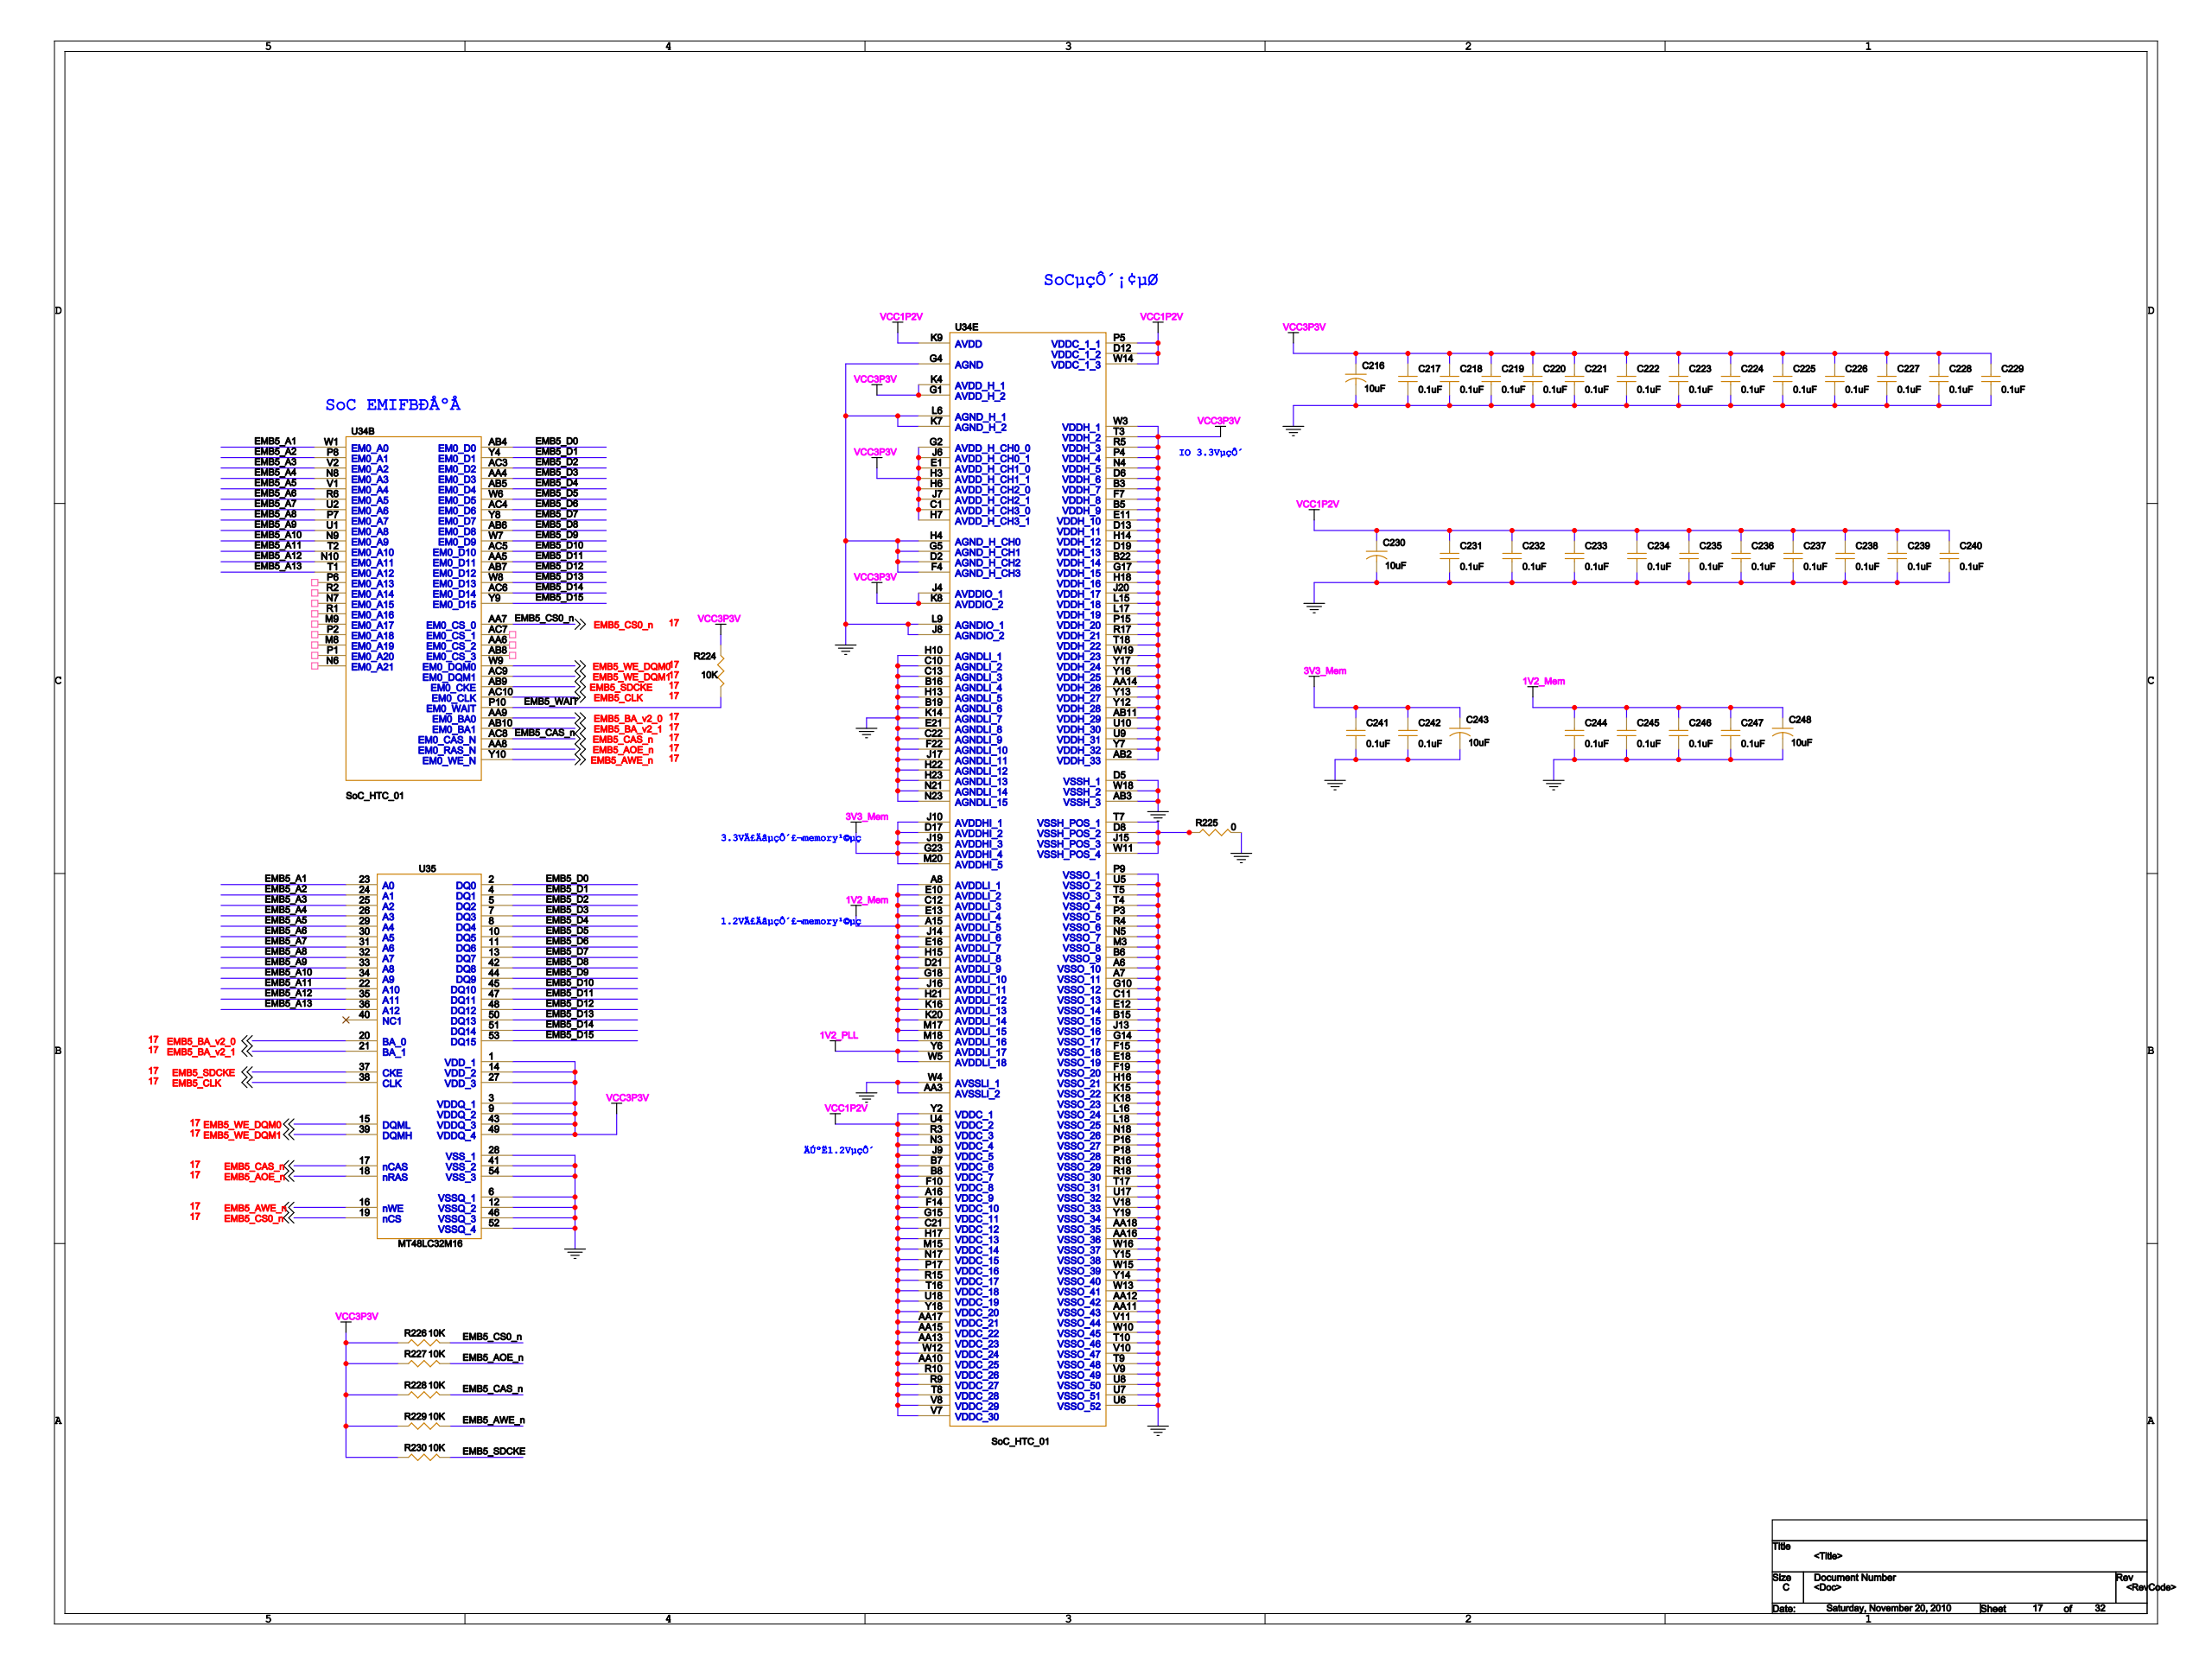Circuit board | Cadence Allegro | 1001 parts | 1318 nets | one sheet of the schematic
Parts on this sheet (reference | value | footprint):
C216 | 10uF | C3216
C217 | 0.1uF | C0402
C218 | 0.1uF | C0402
C219 | 0.1uF | C0402
C220 | 0.1uF | C0402
C221 | 0.1uF | C0402
C222 | 0.1uF | C0402
C223 | 0.1uF | C0402
C224 | 0.1uF | C0402
C225 | 0.1uF | C0402
C226 | 0.1uF | C0402
C227 | 0.1uF | C0402
C228 | 0.1uF | C0402
C229 | 0.1uF | C0402
C230 | 10uF | C3216
C231 | 0.1uF | C0402
C232 | 0.1uF | C0402
C233 | 0.1uF | C0402
C234 | 0.1uF | C0402
C235 | 0.1uF | C0402
C236 | 0.1uF | C0402
C237 | 0.1uF | C0402
C238 | 0.1uF | C0402
C239 | 0.1uF | C0402
C240 | 0.1uF | C0402
C241 | 0.1uF | C0402
C242 | 0.1uF | C0402
C243 | 10uF | C3216
C244 | 0.1uF | C0402
C245 | 0.1uF | C0402
C246 | 0.1uF | C0402
C247 | 0.1uF | C0402
C248 | 10uF | C3216
R224 | 10K | 0603
R225 | 0 | 0603
R226 | 10K | 0603
R227 | 10K | 0603
R228 | 10K | 0603
R229 | 10K | 0603
R230 | 10K | 0603
U1 | SoC_HTC_01 | L529_XIN
U2 | MT48LC32M16 | TSOP54
U4 | MAX3243 | TSSOP-28
U6 | MT48LC16M16 | TSOP54
U7 | MT48LC16M16 | TSOP54
U8 | DP83848C | DP83848C_48LQFP
U10 | SoC_HTC_01 | L529_XIN
U17 | MT48LC32M16 | TSOP54
U34 | SoC_HTC_01 | L529_XIN
U35 | MT48LC32M16 | TSOP54
Nets of these parts (net: part-pin ...):
GND: C216-2 C217-2 C218-2 C219-2 C220-2 C221-2 C222-2 C223-2 C224-2 C225-2 C226-2 C227-2 C228-2 C229-2 C230-2 C231-2 C232-2 C233-2 C234-2 C235-2 C236-2 C237-2 C238-2 C239-2 C240-2 C241-2 C242-2 C243-2 C244-2 C245-2 C246-2 C247-2 C248-2 R225-2 U1-A6 U1-A7 U1-AA3 U1-AA11 U1-AA12 U1-AA16 U1-AA18 U1-AB3 U1-B6 U1-B15 U1-B16 U1-B19 U1-C10 U1-C11 U1-C13 U1-C22 U1-D2 U1-D5 U1-E12 U1-E18 U1-E21 U1-F4 U1-F15 U1-F19 U1-F22 U1-G4 U1-G5 U1-G10 U1-G14 U1-H4 U1-H10 U1-H13 U1-H16 U1-H22 U1-H23 U1-J8 U1-J13 U1-J17 U1-K7 U1-K14 U1-K15 U1-K18 U1-L6 U1-L9 U1-L16 U1-L18 U1-M3 U1-N5 U1-N18 U1-N21 U1-N23 U1-P3 U1-P9 U1-P16 U1-P18 U1-R4 U1-R16 U1-R18 U1-T4 U1-T5 U1-T9 U1-T10 U1-T17 U1-U5 U1-U6 U1-U7 U1-U8 U1-U17 U1-V9 U1-V10 U1-V11 U1-V18 U1-W4 U1-W10 U1-W13 U1-W15 U1-W16 U1-W18 U1-Y14 U1-Y15 U1-Y19 U2-6 U2-12 U2-28 U2-41 U2-46 U2-52 U2-54 U4-23 U4-25 U6-6 U6-12 U6-28 U6-41 U6-46 U6-52 U6-54 U7-6 U7-12 U7-28 U7-41 U7-46 U7-52 U7-54 U8-15 U8-19 U8-35 U8-36 U8-47 U10-A6 U10-A7 U10-AA3 U10-AA11 U10-AA12 U10-AA16 U10-AA18 U10-AB3 U10-B6 U10-B15 U10-B16 U10-B19 U10-C10 U10-C11 U10-C13 U10-C22 U10-D2 U10-D5 U10-E12 U10-E18 U10-E21 U10-F4 U10-F15 U10-F19 U10-F22 U10-G4 U10-G5 U10-G10 U10-G14 U10-H4 U10-H10 U10-H13 U10-H16 U10-H22 U10-H23 U10-J8 U10-J13 U10-J17 U10-K7 U10-K14 U10-K15 U10-K18 U10-L6 U10-L9 U10-L16 U10-L18 U10-M3 U10-N5 U10-N18 U10-N21 U10-N23 U10-P3 U10-P9 U10-P16 U10-P18 U10-R4 U10-R16 U10-R18 U10-T4 U10-T5 U10-T9 U10-T10 U10-T17 U10-U5 U10-U6 U10-U7 U10-U8 U10-U17 U10-V9 U10-V10 U10-V11 U10-V18 U10-W4 U10-W10 U10-W13 U10-W15 U10-W16 U10-W18 U10-Y14 U10-Y15 U10-Y19 U17-6 U17-12 U17-28 U17-41 U17-46 U17-52 U17-54 U34-A6 U34-A7 U34-AA3 U34-AA11 U34-AA12 U34-AA16 U34-AA18 U34-AB3 U34-B6 U34-B15 U34-B16 U34-B19 U34-C10 U34-C11 U34-C13 U34-C22 U34-D2 U34-D5 U34-E12 U34-E18 U34-E21 U34-F4 U34-F15 U34-F19 U34-F22 U34-G4 U34-G5 U34-G10 U34-G14 U34-H4 U34-H10 U34-H13 U34-H16 U34-H22 U34-H23 U34-J8 U34-J13 U34-J17 U34-K7 U34-K14 U34-K15 U34-K18 U34-L6 U34-L9 U34-L16 U34-L18 U34-M3 U34-N5 U34-N18 U34-N21 U34-N23 U34-P3 U34-P9 U34-P16 U34-P18 U34-R4 U34-R16 U34-R18 U34-T4 U34-T5 U34-T9 U34-T10 U34-T17 U34-U5 U34-U6 U34-U7 U34-U8 U34-U17 U34-V9 U34-V10 U34-V11 U34-V18 U34-W4 U34-W10 U34-W13 U34-W15 U34-W16 U34-W18 U34-Y14 U34-Y15 U34-Y19 U35-6 U35-12 U35-28 U35-41 U35-46 U35-52 U35-54
VCC3P3V: C216-1 C217-1 C218-1 C219-1 C220-1 C221-1 C222-1 C223-1 C224-1 C225-1 C226-1 C227-1 C228-1 C229-1 R224-2 R226-1 R227-1 R228-1 R229-1 R230-1 U1-AA14 U1-AB2 U1-AB11 U1-B3 U1-B5 U1-B22 U1-C1 U1-D6 U1-D13 U1-D19 U1-E1 U1-E11 U1-F7 U1-G1 U1-G2 U1-G17 U1-H3 U1-H6 U1-H7 U1-H14 U1-H18 U1-J4 U1-J6 U1-J7 U1-J20 U1-K4 U1-K8 U1-L15 U1-L17 U1-N4 U1-P4 U1-P15 U1-R5 U1-R17 U1-T3 U1-T18 U1-U9 U1-U10 U1-W3 U1-W19 U1-Y7 U1-Y12 U1-Y13 U1-Y16 U1-Y17 U2-1 U2-3 U2-9 U2-14 U2-27 U2-43 U2-49 U4-22 U4-26 U6-1 U6-3 U6-9 U6-14 U6-27 U6-43 U6-49 U7-1 U7-3 U7-9 U7-14 U7-27 U7-43 U7-49 U8-22 U8-32 U8-48 U10-AA14 U10-AB2 U10-AB11 U10-B3 U10-B5 U10-B22 U10-C1 U10-D6 U10-D13 U10-D19 U10-E1 U10-E11 U10-F7 U10-G1 U10-G2 U10-G17 U10-H3 U10-H6 U10-H7 U10-H14 U10-H18 U10-J4 U10-J6 U10-J7 U10-J20 U10-K4 U10-K8 U10-L15 U10-L17 U10-N4 U10-P4 U10-P15 U10-R5 U10-R17 U10-T3 U10-T18 U10-U9 U10-U10 U10-W3 U10-W19 U10-Y7 U10-Y12 U10-Y13 U10-Y16 U10-Y17 U17-1 U17-3 U17-9 U17-14 U17-27 U17-43 U17-49 U34-AA14 U34-AB2 U34-AB11 U34-B3 U34-B5 U34-B22 U34-C1 U34-D6 U34-D13 U34-D19 U34-E1 U34-E11 U34-F7 U34-G1 U34-G2 U34-G17 U34-H3 U34-H6 U34-H7 U34-H14 U34-H18 U34-J4 U34-J6 U34-J7 U34-J20 U34-K4 U34-K8 U34-L15 U34-L17 U34-N4 U34-P4 U34-P15 U34-R5 U34-R17 U34-T3 U34-T18 U34-U9 U34-U10 U34-W3 U34-W19 U34-Y7 U34-Y12 U34-Y13 U34-Y16 U34-Y17 U35-1 U35-3 U35-9 U35-14 U35-27 U35-43 U35-49
VCC1P2V: C230-1 C231-1 C232-1 C233-1 C234-1 C235-1 C236-1 C237-1 C238-1 C239-1 C240-1 U1-A16 U1-AA10 U1-AA13 U1-AA15 U1-AA17 U1-B7 U1-B8 U1-C21 U1-D12 U1-F10 U1-F14 U1-G15 U1-H17 U1-J9 U1-K9 U1-M15 U1-N3 U1-N17 U1-P5 U1-P17 U1-R3 U1-R9 U1-R10 U1-R15 U1-T8 U1-T16 U1-U4 U1-U18 U1-V7 U1-V8 U1-W12 U1-W14 U1-Y2 U1-Y18 U10-A16 U10-AA10 U10-AA13 U10-AA15 U10-AA17 U10-B7 U10-B8 U10-C21 U10-D12 U10-F10 U10-F14 U10-G15 U10-H17 U10-J9 U10-K9 U10-M15 U10-N3 U10-N17 U10-P5 U10-P17 U10-R3 U10-R9 U10-R10 U10-R15 U10-T8 U10-T16 U10-U4 U10-U18 U10-V7 U10-V8 U10-W12 U10-W14 U10-Y2 U10-Y18 U34-A16 U34-AA10 U34-AA13 U34-AA15 U34-AA17 U34-B7 U34-B8 U34-C21 U34-D12 U34-F10 U34-F14 U34-G15 U34-H17 U34-J9 U34-K9 U34-M15 U34-N3 U34-N17 U34-P5 U34-P17 U34-R3 U34-R9 U34-R10 U34-R15 U34-T8 U34-T16 U34-U4 U34-U18 U34-V7 U34-V8 U34-W12 U34-W14 U34-Y2 U34-Y18
3V3_MEM: C241-1 C242-1 C243-1 U1-D17 U1-G23 U1-J10 U1-J19 U1-M20 U10-D17 U10-G23 U10-J10 U10-J19 U10-M20 U34-D17 U34-G23 U34-J10 U34-J19 U34-M20
1V2_MEM: C244-1 C245-1 C246-1 C247-1 C248-1 U1-A8 U1-A15 U1-C12 U1-D21 U1-E10 U1-E13 U1-E16 U1-G18 U1-H15 U1-H21 U1-J14 U1-J16 U1-K16 U1-K20 U1-M17 U1-M18 U10-A8 U10-A15 U10-C12 U10-D21 U10-E10 U10-E13 U10-E16 U10-G18 U10-H15 U10-H21 U10-J14 U10-J16 U10-K16 U10-K20 U10-M17 U10-M18 U34-A8 U34-A15 U34-C12 U34-D21 U34-E10 U34-E13 U34-E16 U34-G18 U34-H15 U34-H21 U34-J14 U34-J16 U34-K16 U34-K20 U34-M17 U34-M18
1V2_PLL: U1-W5 U1-Y6 U10-W5 U10-Y6 U34-W5 U34-Y6
EMB5_A1: U34-W1 U35-23
EMB5_A2: U34-P8 U35-24
EMB5_A11: U34-T2 U35-22
EMB5_A12: U34-N10 U35-35
EMB5_A13: U34-T1 U35-36
EMB5_A3: U34-V2 U35-25
EMB5_A4: U34-N8 U35-26
EMB5_A5: U34-V1 U35-29
EMB5_A6: U34-R6 U35-30
EMB5_A7: U34-U2 U35-31
EMB5_A8: U34-P7 U35-32
EMB5_A9: U34-U1 U35-33
EMB5_A10: U34-N9 U35-34
EMB5_CAS_N: R228-2 U34-AC8 U35-17
EMB5_SDCKE: R230-2 U34-AB9 U35-37
EMB5_CLK: U34-AC10 U35-38
EMB5_CS0_N: R226-2 U34-AA7 U35-19
EMB5_D0: U34-AB4 U35-2
EMB5_D1: U34-Y4 U35-4
EMB5_D10: U34-AC5 U35-45
EMB5_D11: U34-AA5 U35-47
EMB5_D12: U34-AB7 U35-48
EMB5_D13: U34-W8 U35-50
EMB5_D14: U34-AC6 U35-51
EMB5_D15: U34-Y9 U35-53
EMB5_D2: U34-AC3 U35-5
EMB5_D3: U34-AA4 U35-7
EMB5_D4: U34-AB5 U35-8
EMB5_D5: U34-W6 U35-10
EMB5_D6: U34-AC4 U35-11
EMB5_D7: U34-Y8 U35-13
EMB5_D8: U34-AB6 U35-42
EMB5_D9: U34-W7 U35-44
EMB5_WE_DQM0: U34-W9 U35-15
EMB5_WE_DQM1: U34-AC9 U35-39
EMB5_AOE_N: R227-2 U34-AA8 U35-18
EMB5_WAIT: R224-1 U34-P10
EMB5_AWE_N: R229-2 U34-Y10 U35-16
N17411362: R225-1 U34-D8 U34-J15 U34-T7 U34-W11